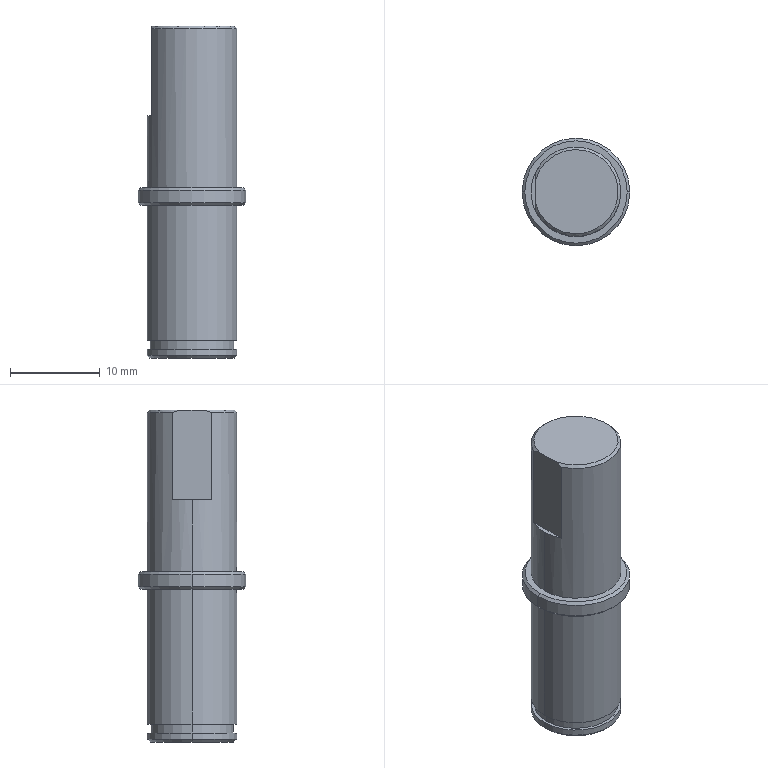Part | SolidWorks | features ICE 3, Chamfer 1, Extrusion 1, RevCut 1 | 1 solid | 25 faces | box 12 x 12 x 37 mm | volume 2944 mm3 | cylinder 10 | plane 8 | cone 7 | commonest cylinder face diameters 10 x6 9.3 x2 12 x2
STEP:
#1=CARTESIAN_POINT('',(-5.7,0.,-2.));
#2=VERTEX_POINT('',#1);
#3=CARTESIAN_POINT('',(5.7,0.,-2.));
#4=VERTEX_POINT('',#3);
#5=CARTESIAN_POINT('',(0.,0.,-2.));
#6=DIRECTION('',(0.,0.,-1.));
#7=DIRECTION('',(-1.,0.,0.));
#8=AXIS2_PLACEMENT_3D('',#5,#6,#7);
#9=CIRCLE('',#8,5.7);
#10=EDGE_CURVE('',#2,#4,#9,.T.);
#11=ORIENTED_EDGE('',*,*,#10,.F.);
#12=CARTESIAN_POINT('',(-6.,0.,-1.7));
#13=VERTEX_POINT('',#12);
#14=CARTESIAN_POINT('',(-5.7,0.,-2.));
#15=DIRECTION('',(-0.7071,0.,0.7071));
#16=VECTOR('',#15,1000.);
#17=LINE('',#14,#16);
#18=EDGE_CURVE('',#2,#13,#17,.T.);
#19=ORIENTED_EDGE('',*,*,#18,.T.);
#20=CARTESIAN_POINT('',(6.,0.,-1.7));
#21=VERTEX_POINT('',#20);
#22=CARTESIAN_POINT('',(0.,0.,-1.7));
#23=DIRECTION('',(0.,0.,1.));
#24=DIRECTION('',(-1.,0.,0.));
#25=AXIS2_PLACEMENT_3D('',#22,#23,#24);
#26=CIRCLE('',#25,6.);
#27=EDGE_CURVE('',#21,#13,#26,.T.);
#28=ORIENTED_EDGE('',*,*,#27,.F.);
#29=CARTESIAN_POINT('',(5.7,0.,-2.));
#30=DIRECTION('',(0.7071,0.,0.7071));
#31=VECTOR('',#30,1000.);
#32=LINE('',#29,#31);
#33=EDGE_CURVE('',#4,#21,#32,.T.);
#34=ORIENTED_EDGE('',*,*,#33,.F.);
#35=EDGE_LOOP('',(#11,#19,#28,#34));
#36=FACE_OUTER_BOUND('',#35,.T.);
#37=CARTESIAN_POINT('',(0.,0.,-2.));
#38=DIRECTION('',(0.,0.,1.));
#39=DIRECTION('',(1.,0.,0.));
#40=AXIS2_PLACEMENT_3D('',#37,#38,#39);
#41=CONICAL_SURFACE('',#40,5.7,0.7854);
#42=ADVANCED_FACE('',(#36),#41,.T.);
#43=CARTESIAN_POINT('',(5.7,0.,0.));
#44=VERTEX_POINT('',#43);
#45=CARTESIAN_POINT('',(-5.7,0.,0.));
#46=VERTEX_POINT('',#45);
#47=CARTESIAN_POINT('',(0.,0.,0.));
#48=DIRECTION('',(0.,0.,1.));
#49=DIRECTION('',(-1.,0.,0.));
#50=AXIS2_PLACEMENT_3D('',#47,#48,#49);
#51=CIRCLE('',#50,5.7);
#52=EDGE_CURVE('',#44,#46,#51,.T.);
#53=ORIENTED_EDGE('',*,*,#52,.F.);
#54=CARTESIAN_POINT('',(6.,0.,-0.3));
#55=VERTEX_POINT('',#54);
#56=CARTESIAN_POINT('',(6.,0.,-0.3));
#57=DIRECTION('',(0.7071,0.,-0.7071));
#58=VECTOR('',#57,1000.);
#59=LINE('',#56,#58);
#60=EDGE_CURVE('',#44,#55,#59,.T.);
#61=ORIENTED_EDGE('',*,*,#60,.T.);
#62=CARTESIAN_POINT('',(-6.,0.,-0.3));
#63=VERTEX_POINT('',#62);
#64=CARTESIAN_POINT('',(0.,0.,-0.3));
#65=DIRECTION('',(0.,0.,-1.));
#66=DIRECTION('',(-1.,0.,0.));
#67=AXIS2_PLACEMENT_3D('',#64,#65,#66);
#68=CIRCLE('',#67,6.);
#69=EDGE_CURVE('',#63,#55,#68,.T.);
#70=ORIENTED_EDGE('',*,*,#69,.F.);
#71=CARTESIAN_POINT('',(-6.,0.,-0.3));
#72=DIRECTION('',(-0.7071,0.,-0.7071));
#73=VECTOR('',#72,1000.);
#74=LINE('',#71,#73);
#75=EDGE_CURVE('',#46,#63,#74,.T.);
#76=ORIENTED_EDGE('',*,*,#75,.F.);
#77=EDGE_LOOP('',(#53,#61,#70,#76));
#78=FACE_OUTER_BOUND('',#77,.T.);
#79=CARTESIAN_POINT('',(0.,0.,-0.3));
#80=DIRECTION('',(0.,0.,-1.));
#81=DIRECTION('',(-1.,0.,0.));
#82=AXIS2_PLACEMENT_3D('',#79,#80,#81);
#83=CONICAL_SURFACE('',#82,6.,0.7854);
#84=ADVANCED_FACE('',(#78),#83,.T.);
#85=CARTESIAN_POINT('',(-4.7,0.,-19.));
#86=VERTEX_POINT('',#85);
#87=CARTESIAN_POINT('',(4.7,0.,-19.));
#88=VERTEX_POINT('',#87);
#89=CARTESIAN_POINT('',(0.,0.,-19.));
#90=DIRECTION('',(0.,0.,-1.));
#91=DIRECTION('',(-1.,0.,0.));
#92=AXIS2_PLACEMENT_3D('',#89,#90,#91);
#93=CIRCLE('',#92,4.7);
#94=EDGE_CURVE('',#86,#88,#93,.T.);
#95=ORIENTED_EDGE('',*,*,#94,.F.);
#96=CARTESIAN_POINT('',(-5.,0.,-18.7));
#97=VERTEX_POINT('',#96);
#98=CARTESIAN_POINT('',(-4.7,0.,-19.));
#99=DIRECTION('',(-0.7071,0.,0.7071));
#100=VECTOR('',#99,1000.);
#101=LINE('',#98,#100);
#102=EDGE_CURVE('',#86,#97,#101,.T.);
#103=ORIENTED_EDGE('',*,*,#102,.T.);
#104=CARTESIAN_POINT('',(5.,0.,-18.7));
#105=VERTEX_POINT('',#104);
#106=CARTESIAN_POINT('',(0.,0.,-18.7));
#107=DIRECTION('',(0.,0.,1.));
#108=DIRECTION('',(-1.,0.,0.));
#109=AXIS2_PLACEMENT_3D('',#106,#107,#108);
#110=CIRCLE('',#109,5.);
#111=EDGE_CURVE('',#105,#97,#110,.T.);
#112=ORIENTED_EDGE('',*,*,#111,.F.);
#113=CARTESIAN_POINT('',(4.7,0.,-19.));
#114=DIRECTION('',(0.7071,0.,0.7071));
#115=VECTOR('',#114,1000.);
#116=LINE('',#113,#115);
#117=EDGE_CURVE('',#88,#105,#116,.T.);
#118=ORIENTED_EDGE('',*,*,#117,.F.);
#119=EDGE_LOOP('',(#95,#103,#112,#118));
#120=FACE_OUTER_BOUND('',#119,.T.);
#121=CARTESIAN_POINT('',(0.,0.,-19.));
#122=DIRECTION('',(0.,0.,1.));
#123=DIRECTION('',(1.,0.,0.));
#124=AXIS2_PLACEMENT_3D('',#121,#122,#123);
#125=CONICAL_SURFACE('',#124,4.7,0.7854);
#126=ADVANCED_FACE('',(#120),#125,.T.);
#127=ORIENTED_EDGE('',*,*,#111,.T.);
#128=CARTESIAN_POINT('',(-5.,0.,-18.));
#129=VERTEX_POINT('',#128);
#130=CARTESIAN_POINT('',(-5.,0.,-19.));
#131=DIRECTION('',(0.,0.,1.));
#132=VECTOR('',#131,1000.);
#133=LINE('',#130,#132);
#134=EDGE_CURVE('',#97,#129,#133,.T.);
#135=ORIENTED_EDGE('',*,*,#134,.T.);
#136=CARTESIAN_POINT('',(5.,0.,-18.));
#137=VERTEX_POINT('',#136);
#138=CARTESIAN_POINT('',(0.,0.,-18.));
#139=DIRECTION('',(0.,0.,-1.));
#140=DIRECTION('',(-1.,0.,0.));
#141=AXIS2_PLACEMENT_3D('',#138,#139,#140);
#142=CIRCLE('',#141,5.);
#143=EDGE_CURVE('',#129,#137,#142,.T.);
#144=ORIENTED_EDGE('',*,*,#143,.T.);
#145=CARTESIAN_POINT('',(5.,0.,-19.));
#146=DIRECTION('',(0.,0.,1.));
#147=VECTOR('',#146,1000.);
#148=LINE('',#145,#147);
#149=EDGE_CURVE('',#105,#137,#148,.T.);
#150=ORIENTED_EDGE('',*,*,#149,.F.);
#151=EDGE_LOOP('',(#127,#135,#144,#150));
#152=FACE_OUTER_BOUND('',#151,.T.);
#153=CARTESIAN_POINT('',(0.,0.,-19.));
#154=DIRECTION('',(0.,0.,1.));
#155=DIRECTION('',(1.,0.,0.));
#156=AXIS2_PLACEMENT_3D('',#153,#154,#155);
#157=CYLINDRICAL_SURFACE('',#156,5.);
#158=ADVANCED_FACE('',(#152),#157,.T.);
#159=CARTESIAN_POINT('',(-4.65,0.,-17.));
#160=VERTEX_POINT('',#159);
#161=CARTESIAN_POINT('',(4.65,0.,-17.));
#162=VERTEX_POINT('',#161);
#163=CARTESIAN_POINT('',(0.,0.,-17.));
#164=DIRECTION('',(0.,0.,-1.));
#165=DIRECTION('',(-1.,0.,0.));
#166=AXIS2_PLACEMENT_3D('',#163,#164,#165);
#167=CIRCLE('',#166,4.65);
#168=EDGE_CURVE('',#160,#162,#167,.T.);
#169=ORIENTED_EDGE('',*,*,#168,.T.);
#170=CARTESIAN_POINT('',(4.65,0.,-18.));
#171=VERTEX_POINT('',#170);
#172=CARTESIAN_POINT('',(4.65,0.,-19.));
#173=DIRECTION('',(0.,0.,-1.));
#174=VECTOR('',#173,1000.);
#175=LINE('',#172,#174);
#176=EDGE_CURVE('',#162,#171,#175,.T.);
#177=ORIENTED_EDGE('',*,*,#176,.T.);
#178=CARTESIAN_POINT('',(-4.65,0.,-18.));
#179=VERTEX_POINT('',#178);
#180=CARTESIAN_POINT('',(0.,0.,-18.));
#181=DIRECTION('',(0.,0.,-1.));
#182=DIRECTION('',(-1.,0.,0.));
#183=AXIS2_PLACEMENT_3D('',#180,#181,#182);
#184=CIRCLE('',#183,4.65);
#185=EDGE_CURVE('',#179,#171,#184,.T.);
#186=ORIENTED_EDGE('',*,*,#185,.F.);
#187=CARTESIAN_POINT('',(-4.65,0.,-19.));
#188=DIRECTION('',(0.,0.,-1.));
#189=VECTOR('',#188,1000.);
#190=LINE('',#187,#189);
#191=EDGE_CURVE('',#160,#179,#190,.T.);
#192=ORIENTED_EDGE('',*,*,#191,.F.);
#193=EDGE_LOOP('',(#169,#177,#186,#192));
#194=FACE_OUTER_BOUND('',#193,.T.);
#195=CARTESIAN_POINT('',(0.,0.,-19.));
#196=DIRECTION('',(0.,0.,-1.));
#197=DIRECTION('',(-1.,0.,0.));
#198=AXIS2_PLACEMENT_3D('',#195,#196,#197);
#199=CYLINDRICAL_SURFACE('',#198,4.65);
#200=ADVANCED_FACE('',(#194),#199,.T.);
#201=ORIENTED_EDGE('',*,*,#27,.T.);
#202=CARTESIAN_POINT('',(-6.,0.,-2.));
#203=DIRECTION('',(0.,0.,1.));
#204=VECTOR('',#203,1000.);
#205=LINE('',#202,#204);
#206=EDGE_CURVE('',#13,#63,#205,.T.);
#207=ORIENTED_EDGE('',*,*,#206,.T.);
#208=ORIENTED_EDGE('',*,*,#69,.T.);
#209=CARTESIAN_POINT('',(6.,0.,-2.));
#210=DIRECTION('',(0.,0.,1.));
#211=VECTOR('',#210,1000.);
#212=LINE('',#209,#211);
#213=EDGE_CURVE('',#21,#55,#212,.T.);
#214=ORIENTED_EDGE('',*,*,#213,.F.);
#215=EDGE_LOOP('',(#201,#207,#208,#214));
#216=FACE_OUTER_BOUND('',#215,.T.);
#217=CARTESIAN_POINT('',(0.,0.,-2.));
#218=DIRECTION('',(0.,0.,1.));
#219=DIRECTION('',(1.,0.,0.));
#220=AXIS2_PLACEMENT_3D('',#217,#218,#219);
#221=CYLINDRICAL_SURFACE('',#220,6.);
#222=ADVANCED_FACE('',(#216),#221,.T.);
#223=CARTESIAN_POINT('',(5.,0.,-17.));
#224=VERTEX_POINT('',#223);
#225=CARTESIAN_POINT('',(-5.,0.,-17.));
#226=VERTEX_POINT('',#225);
#227=CARTESIAN_POINT('',(0.,0.,-17.));
#228=DIRECTION('',(0.,0.,1.));
#229=DIRECTION('',(1.,0.,0.));
#230=AXIS2_PLACEMENT_3D('',#227,#228,#229);
#231=CIRCLE('',#230,5.);
#232=EDGE_CURVE('',#224,#226,#231,.T.);
#233=ORIENTED_EDGE('',*,*,#232,.T.);
#234=CARTESIAN_POINT('',(-5.,0.,-2.));
#235=VERTEX_POINT('',#234);
#236=CARTESIAN_POINT('',(-5.,0.,-19.));
#237=DIRECTION('',(0.,0.,1.));
#238=VECTOR('',#237,1000.);
#239=LINE('',#236,#238);
#240=EDGE_CURVE('',#226,#235,#239,.T.);
#241=ORIENTED_EDGE('',*,*,#240,.T.);
#242=CARTESIAN_POINT('',(5.,0.,-2.));
#243=VERTEX_POINT('',#242);
#244=CARTESIAN_POINT('',(0.,0.,-2.));
#245=DIRECTION('',(0.,0.,-1.));
#246=DIRECTION('',(-1.,0.,0.));
#247=AXIS2_PLACEMENT_3D('',#244,#245,#246);
#248=CIRCLE('',#247,5.);
#249=EDGE_CURVE('',#235,#243,#248,.T.);
#250=ORIENTED_EDGE('',*,*,#249,.T.);
#251=CARTESIAN_POINT('',(5.,0.,-19.));
#252=DIRECTION('',(0.,0.,1.));
#253=VECTOR('',#252,1000.);
#254=LINE('',#251,#253);
#255=EDGE_CURVE('',#224,#243,#254,.T.);
#256=ORIENTED_EDGE('',*,*,#255,.F.);
#257=EDGE_LOOP('',(#233,#241,#250,#256));
#258=FACE_OUTER_BOUND('',#257,.T.);
#259=CARTESIAN_POINT('',(0.,0.,-19.));
#260=DIRECTION('',(0.,0.,1.));
#261=DIRECTION('',(1.,0.,0.));
#262=AXIS2_PLACEMENT_3D('',#259,#260,#261);
#263=CYLINDRICAL_SURFACE('',#262,5.);
#264=ADVANCED_FACE('',(#258),#263,.T.);
#265=CARTESIAN_POINT('',(-4.5,2.179,17.7));
#266=VERTEX_POINT('',#265);
#267=CARTESIAN_POINT('',(5.,0.,17.7));
#268=VERTEX_POINT('',#267);
#269=CARTESIAN_POINT('',(0.,0.,17.7));
#270=DIRECTION('',(0.,0.,-1.));
#271=DIRECTION('',(1.,0.,0.));
#272=AXIS2_PLACEMENT_3D('',#269,#270,#271);
#273=CIRCLE('',#272,5.);
#274=EDGE_CURVE('',#266,#268,#273,.T.);
#275=ORIENTED_EDGE('',*,*,#274,.T.);
#276=CARTESIAN_POINT('',(5.,0.,0.));
#277=VERTEX_POINT('',#276);
#278=CARTESIAN_POINT('',(5.,0.,18.));
#279=DIRECTION('',(0.,0.,-1.));
#280=VECTOR('',#279,1000.);
#281=LINE('',#278,#280);
#282=EDGE_CURVE('',#268,#277,#281,.T.);
#283=ORIENTED_EDGE('',*,*,#282,.T.);
#284=CARTESIAN_POINT('',(-5.,0.,0.));
#285=VERTEX_POINT('',#284);
#286=CARTESIAN_POINT('',(0.,0.,0.));
#287=DIRECTION('',(0.,0.,-1.));
#288=DIRECTION('',(-1.,0.,0.));
#289=AXIS2_PLACEMENT_3D('',#286,#287,#288);
#290=CIRCLE('',#289,5.);
#291=EDGE_CURVE('',#285,#277,#290,.T.);
#292=ORIENTED_EDGE('',*,*,#291,.F.);
#293=CARTESIAN_POINT('',(-5.,0.,8.));
#294=VERTEX_POINT('',#293);
#295=CARTESIAN_POINT('',(-5.,0.,18.));
#296=DIRECTION('',(0.,0.,-1.));
#297=VECTOR('',#296,1000.);
#298=LINE('',#295,#297);
#299=EDGE_CURVE('',#294,#285,#298,.T.);
#300=ORIENTED_EDGE('',*,*,#299,.F.);
#301=CARTESIAN_POINT('',(-4.5,2.179,8.));
#302=VERTEX_POINT('',#301);
#303=CARTESIAN_POINT('',(0.,0.,8.));
#304=DIRECTION('',(0.,0.,1.));
#305=DIRECTION('',(1.,0.,0.));
#306=AXIS2_PLACEMENT_3D('',#303,#304,#305);
#307=CIRCLE('',#306,5.);
#308=EDGE_CURVE('',#302,#294,#307,.T.);
#309=ORIENTED_EDGE('',*,*,#308,.F.);
#310=CARTESIAN_POINT('',(-4.5,2.179,18.));
#311=DIRECTION('',(0.,0.,-1.));
#312=VECTOR('',#311,1000.);
#313=LINE('',#310,#312);
#314=EDGE_CURVE('',#266,#302,#313,.T.);
#315=ORIENTED_EDGE('',*,*,#314,.F.);
#316=EDGE_LOOP('',(#275,#283,#292,#300,#309,#315));
#317=FACE_OUTER_BOUND('',#316,.T.);
#318=CARTESIAN_POINT('',(0.,0.,18.));
#319=DIRECTION('',(0.,0.,-1.));
#320=DIRECTION('',(-1.,0.,0.));
#321=AXIS2_PLACEMENT_3D('',#318,#319,#320);
#322=CYLINDRICAL_SURFACE('',#321,5.);
#323=ADVANCED_FACE('',(#317),#322,.T.);
#324=ORIENTED_EDGE('',*,*,#282,.F.);
#325=CARTESIAN_POINT('',(-4.5,-2.179,17.7));
#326=VERTEX_POINT('',#325);
#327=CARTESIAN_POINT('',(0.,0.,17.7));
#328=DIRECTION('',(0.,0.,-1.));
#329=DIRECTION('',(1.,0.,0.));
#330=AXIS2_PLACEMENT_3D('',#327,#328,#329);
#331=CIRCLE('',#330,5.);
#332=EDGE_CURVE('',#268,#326,#331,.T.);
#333=ORIENTED_EDGE('',*,*,#332,.T.);
#334=CARTESIAN_POINT('',(-4.5,-2.179,8.));
#335=VERTEX_POINT('',#334);
#336=CARTESIAN_POINT('',(-4.5,-2.179,18.));
#337=DIRECTION('',(0.,0.,1.));
#338=VECTOR('',#337,1000.);
#339=LINE('',#336,#338);
#340=EDGE_CURVE('',#335,#326,#339,.T.);
#341=ORIENTED_EDGE('',*,*,#340,.F.);
#342=CARTESIAN_POINT('',(0.,0.,8.));
#343=DIRECTION('',(0.,0.,1.));
#344=DIRECTION('',(1.,0.,0.));
#345=AXIS2_PLACEMENT_3D('',#342,#343,#344);
#346=CIRCLE('',#345,5.);
#347=EDGE_CURVE('',#294,#335,#346,.T.);
#348=ORIENTED_EDGE('',*,*,#347,.F.);
#349=ORIENTED_EDGE('',*,*,#299,.T.);
#350=CARTESIAN_POINT('',(0.,0.,0.));
#351=DIRECTION('',(0.,0.,-1.));
#352=DIRECTION('',(-1.,0.,0.));
#353=AXIS2_PLACEMENT_3D('',#350,#351,#352);
#354=CIRCLE('',#353,5.);
#355=EDGE_CURVE('',#277,#285,#354,.T.);
#356=ORIENTED_EDGE('',*,*,#355,.F.);
#357=EDGE_LOOP('',(#324,#333,#341,#348,#349,#356));
#358=FACE_OUTER_BOUND('',#357,.T.);
#359=CARTESIAN_POINT('',(0.,0.,18.));
#360=DIRECTION('',(0.,0.,-1.));
#361=DIRECTION('',(-1.,0.,0.));
#362=AXIS2_PLACEMENT_3D('',#359,#360,#361);
#363=CYLINDRICAL_SURFACE('',#362,5.);
#364=ADVANCED_FACE('',(#358),#363,.T.);
#365=CARTESIAN_POINT('',(-4.5,1.356,18.));
#366=VERTEX_POINT('',#365);
#367=CARTESIAN_POINT('',(-4.5,-1.356,18.));
#368=VERTEX_POINT('',#367);
#369=CARTESIAN_POINT('',(-4.5,0.,18.));
#370=DIRECTION('',(0.,-1.,0.));
#371=VECTOR('',#370,1000.);
#372=LINE('',#369,#371);
#373=EDGE_CURVE('',#366,#368,#372,.T.);
#374=ORIENTED_EDGE('',*,*,#373,.T.);
#375=CARTESIAN_POINT('',(0.,0.,18.));
#376=DIRECTION('',(0.,0.,1.));
#377=DIRECTION('',(1.,0.,0.));
#378=AXIS2_PLACEMENT_3D('',#375,#376,#377);
#379=CIRCLE('',#378,4.7);
#380=EDGE_CURVE('',#368,#366,#379,.T.);
#381=ORIENTED_EDGE('',*,*,#380,.T.);
#382=EDGE_LOOP('',(#374,#381));
#383=FACE_OUTER_BOUND('',#382,.T.);
#384=CARTESIAN_POINT('',(0.,0.,18.));
#385=DIRECTION('',(0.,0.,1.));
#386=DIRECTION('',(1.,0.,0.));
#387=AXIS2_PLACEMENT_3D('',#384,#385,#386);
#388=PLANE('',#387);
#389=ADVANCED_FACE('',(#383),#388,.T.);
#390=ORIENTED_EDGE('',*,*,#240,.F.);
#391=CARTESIAN_POINT('',(0.,0.,-17.));
#392=DIRECTION('',(0.,0.,1.));
#393=DIRECTION('',(1.,0.,0.));
#394=AXIS2_PLACEMENT_3D('',#391,#392,#393);
#395=CIRCLE('',#394,5.);
#396=EDGE_CURVE('',#226,#224,#395,.T.);
#397=ORIENTED_EDGE('',*,*,#396,.T.);
#398=ORIENTED_EDGE('',*,*,#255,.T.);
#399=CARTESIAN_POINT('',(0.,0.,-2.));
#400=DIRECTION('',(0.,0.,-1.));
#401=DIRECTION('',(-1.,0.,0.));
#402=AXIS2_PLACEMENT_3D('',#399,#400,#401);
#403=CIRCLE('',#402,5.);
#404=EDGE_CURVE('',#243,#235,#403,.T.);
#405=ORIENTED_EDGE('',*,*,#404,.T.);
#406=EDGE_LOOP('',(#390,#397,#398,#405));
#407=FACE_OUTER_BOUND('',#406,.T.);
#408=CARTESIAN_POINT('',(0.,0.,-19.));
#409=DIRECTION('',(0.,0.,1.));
#410=DIRECTION('',(1.,0.,0.));
#411=AXIS2_PLACEMENT_3D('',#408,#409,#410);
#412=CYLINDRICAL_SURFACE('',#411,5.);
#413=ADVANCED_FACE('',(#407),#412,.T.);
#414=CARTESIAN_POINT('',(0.,0.,-2.));
#415=DIRECTION('',(0.,0.,-1.));
#416=DIRECTION('',(-1.,0.,0.));
#417=AXIS2_PLACEMENT_3D('',#414,#415,#416);
#418=CIRCLE('',#417,5.7);
#419=EDGE_CURVE('',#4,#2,#418,.T.);
#420=ORIENTED_EDGE('',*,*,#419,.T.);
#421=ORIENTED_EDGE('',*,*,#10,.T.);
#422=EDGE_LOOP('',(#420,#421));
#423=FACE_OUTER_BOUND('',#422,.T.);
#424=ORIENTED_EDGE('',*,*,#404,.F.);
#425=ORIENTED_EDGE('',*,*,#249,.F.);
#426=EDGE_LOOP('',(#424,#425));
#427=FACE_BOUND('',#426,.T.);
#428=CARTESIAN_POINT('',(0.,0.,-2.));
#429=DIRECTION('',(0.,0.,-1.));
#430=DIRECTION('',(-1.,0.,0.));
#431=AXIS2_PLACEMENT_3D('',#428,#429,#430);
#432=PLANE('',#431);
#433=ADVANCED_FACE('',(#423,#427),#432,.T.);
#434=CARTESIAN_POINT('',(0.,0.,0.));
#435=DIRECTION('',(0.,0.,1.));
#436=DIRECTION('',(-1.,0.,0.));
#437=AXIS2_PLACEMENT_3D('',#434,#435,#436);
#438=CIRCLE('',#437,5.7);
#439=EDGE_CURVE('',#46,#44,#438,.T.);
#440=ORIENTED_EDGE('',*,*,#439,.T.);
#441=ORIENTED_EDGE('',*,*,#52,.T.);
#442=EDGE_LOOP('',(#440,#441));
#443=FACE_OUTER_BOUND('',#442,.T.);
#444=ORIENTED_EDGE('',*,*,#291,.T.);
#445=ORIENTED_EDGE('',*,*,#355,.T.);
#446=EDGE_LOOP('',(#444,#445));
#447=FACE_BOUND('',#446,.T.);
#448=CARTESIAN_POINT('',(0.,0.,0.));
#449=DIRECTION('',(0.,0.,-1.));
#450=DIRECTION('',(-1.,0.,0.));
#451=AXIS2_PLACEMENT_3D('',#448,#449,#450);
#452=PLANE('',#451);
#453=ADVANCED_FACE('',(#443,#447),#452,.F.);
#454=ORIENTED_EDGE('',*,*,#206,.F.);
#455=CARTESIAN_POINT('',(0.,0.,-1.7));
#456=DIRECTION('',(0.,0.,1.));
#457=DIRECTION('',(-1.,0.,0.));
#458=AXIS2_PLACEMENT_3D('',#455,#456,#457);
#459=CIRCLE('',#458,6.);
#460=EDGE_CURVE('',#13,#21,#459,.T.);
#461=ORIENTED_EDGE('',*,*,#460,.T.);
#462=ORIENTED_EDGE('',*,*,#213,.T.);
#463=CARTESIAN_POINT('',(0.,0.,-0.3));
#464=DIRECTION('',(0.,0.,-1.));
#465=DIRECTION('',(-1.,0.,0.));
#466=AXIS2_PLACEMENT_3D('',#463,#464,#465);
#467=CIRCLE('',#466,6.);
#468=EDGE_CURVE('',#55,#63,#467,.T.);
#469=ORIENTED_EDGE('',*,*,#468,.T.);
#470=EDGE_LOOP('',(#454,#461,#462,#469));
#471=FACE_OUTER_BOUND('',#470,.T.);
#472=CARTESIAN_POINT('',(0.,0.,-2.));
#473=DIRECTION('',(0.,0.,1.));
#474=DIRECTION('',(1.,0.,0.));
#475=AXIS2_PLACEMENT_3D('',#472,#473,#474);
#476=CYLINDRICAL_SURFACE('',#475,6.);
#477=ADVANCED_FACE('',(#471),#476,.T.);
#478=ORIENTED_EDGE('',*,*,#168,.F.);
#479=CARTESIAN_POINT('',(0.,0.,-17.));
#480=DIRECTION('',(0.,0.,-1.));
#481=DIRECTION('',(-1.,0.,0.));
#482=AXIS2_PLACEMENT_3D('',#479,#480,#481);
#483=CIRCLE('',#482,4.65);
#484=EDGE_CURVE('',#162,#160,#483,.T.);
#485=ORIENTED_EDGE('',*,*,#484,.F.);
#486=EDGE_LOOP('',(#478,#485));
#487=FACE_BOUND('',#486,.T.);
#488=ORIENTED_EDGE('',*,*,#232,.F.);
#489=ORIENTED_EDGE('',*,*,#396,.F.);
#490=EDGE_LOOP('',(#488,#489));
#491=FACE_OUTER_BOUND('',#490,.T.);
#492=CARTESIAN_POINT('',(-6.629,0.,-17.));
#493=DIRECTION('',(0.,0.,1.));
#494=DIRECTION('',(1.,0.,0.));
#495=AXIS2_PLACEMENT_3D('',#492,#493,#494);
#496=PLANE('',#495);
#497=ADVANCED_FACE('',(#487,#491),#496,.F.);
#498=ORIENTED_EDGE('',*,*,#185,.T.);
#499=CARTESIAN_POINT('',(0.,0.,-18.));
#500=DIRECTION('',(0.,0.,-1.));
#501=DIRECTION('',(-1.,0.,0.));
#502=AXIS2_PLACEMENT_3D('',#499,#500,#501);
#503=CIRCLE('',#502,4.65);
#504=EDGE_CURVE('',#171,#179,#503,.T.);
#505=ORIENTED_EDGE('',*,*,#504,.T.);
#506=EDGE_LOOP('',(#498,#505));
#507=FACE_BOUND('',#506,.T.);
#508=CARTESIAN_POINT('',(0.,0.,-18.));
#509=DIRECTION('',(0.,0.,-1.));
#510=DIRECTION('',(-1.,0.,0.));
#511=AXIS2_PLACEMENT_3D('',#508,#509,#510);
#512=CIRCLE('',#511,5.);
#513=EDGE_CURVE('',#137,#129,#512,.T.);
#514=ORIENTED_EDGE('',*,*,#513,.F.);
#515=ORIENTED_EDGE('',*,*,#143,.F.);
#516=EDGE_LOOP('',(#514,#515));
#517=FACE_OUTER_BOUND('',#516,.T.);
#518=CARTESIAN_POINT('',(-6.629,0.,-18.));
#519=DIRECTION('',(0.,0.,-1.));
#520=DIRECTION('',(-1.,0.,0.));
#521=AXIS2_PLACEMENT_3D('',#518,#519,#520);
#522=PLANE('',#521);
#523=ADVANCED_FACE('',(#507,#517),#522,.F.);
#524=ORIENTED_EDGE('',*,*,#176,.F.);
#525=ORIENTED_EDGE('',*,*,#484,.T.);
#526=ORIENTED_EDGE('',*,*,#191,.T.);
#527=ORIENTED_EDGE('',*,*,#504,.F.);
#528=EDGE_LOOP('',(#524,#525,#526,#527));
#529=FACE_OUTER_BOUND('',#528,.T.);
#530=CARTESIAN_POINT('',(0.,0.,-19.));
#531=DIRECTION('',(0.,0.,-1.));
#532=DIRECTION('',(-1.,0.,0.));
#533=AXIS2_PLACEMENT_3D('',#530,#531,#532);
#534=CYLINDRICAL_SURFACE('',#533,4.65);
#535=ADVANCED_FACE('',(#529),#534,.T.);
#536=CARTESIAN_POINT('',(0.,0.,-19.));
#537=DIRECTION('',(0.,0.,-1.));
#538=DIRECTION('',(-1.,0.,0.));
#539=AXIS2_PLACEMENT_3D('',#536,#537,#538);
#540=CIRCLE('',#539,4.7);
#541=EDGE_CURVE('',#88,#86,#540,.T.);
#542=ORIENTED_EDGE('',*,*,#541,.T.);
#543=ORIENTED_EDGE('',*,*,#94,.T.);
#544=EDGE_LOOP('',(#542,#543));
#545=FACE_OUTER_BOUND('',#544,.T.);
#546=CARTESIAN_POINT('',(0.,0.,-19.));
#547=DIRECTION('',(0.,0.,-1.));
#548=DIRECTION('',(-1.,0.,0.));
#549=AXIS2_PLACEMENT_3D('',#546,#547,#548);
#550=PLANE('',#549);
#551=ADVANCED_FACE('',(#545),#550,.T.);
#552=ORIENTED_EDGE('',*,*,#134,.F.);
#553=CARTESIAN_POINT('',(0.,0.,-18.7));
#554=DIRECTION('',(0.,0.,1.));
#555=DIRECTION('',(-1.,0.,0.));
#556=AXIS2_PLACEMENT_3D('',#553,#554,#555);
#557=CIRCLE('',#556,5.);
#558=EDGE_CURVE('',#97,#105,#557,.T.);
#559=ORIENTED_EDGE('',*,*,#558,.T.);
#560=ORIENTED_EDGE('',*,*,#149,.T.);
#561=ORIENTED_EDGE('',*,*,#513,.T.);
#562=EDGE_LOOP('',(#552,#559,#560,#561));
#563=FACE_OUTER_BOUND('',#562,.T.);
#564=CARTESIAN_POINT('',(0.,0.,-19.));
#565=DIRECTION('',(0.,0.,1.));
#566=DIRECTION('',(1.,0.,0.));
#567=AXIS2_PLACEMENT_3D('',#564,#565,#566);
#568=CYLINDRICAL_SURFACE('',#567,5.);
#569=ADVANCED_FACE('',(#563),#568,.T.);
#570=ORIENTED_EDGE('',*,*,#308,.T.);
#571=ORIENTED_EDGE('',*,*,#347,.T.);
#572=CARTESIAN_POINT('',(-4.5,10.,8.));
#573=DIRECTION('',(0.,-1.,0.));
#574=VECTOR('',#573,1000.);
#575=LINE('',#572,#574);
#576=EDGE_CURVE('',#302,#335,#575,.T.);
#577=ORIENTED_EDGE('',*,*,#576,.F.);
#578=EDGE_LOOP('',(#570,#571,#577));
#579=FACE_OUTER_BOUND('',#578,.T.);
#580=CARTESIAN_POINT('',(-10.067,10.,8.));
#581=DIRECTION('',(0.,0.,1.));
#582=DIRECTION('',(1.,0.,0.));
#583=AXIS2_PLACEMENT_3D('',#580,#581,#582);
#584=PLANE('',#583);
#585=ADVANCED_FACE('',(#579),#584,.T.);
#586=ORIENTED_EDGE('',*,*,#373,.F.);
#587=CARTESIAN_POINT('',(-4.5,1.356,18.));
#588=CARTESIAN_POINT('',(-4.5,1.638,17.919));
#589=CARTESIAN_POINT('',(-4.5,1.911,17.817));
#590=CARTESIAN_POINT('',(-4.5,2.179,17.7));
#591=B_SPLINE_CURVE_WITH_KNOTS('',3,(#587,#588,#589,#590),.UNSPECIFIED.,.F.,.F.,(4,4),(0.,0.000876),.UNSPECIFIED.);
#592=EDGE_CURVE('',#366,#266,#591,.T.);
#593=ORIENTED_EDGE('',*,*,#592,.T.);
#594=ORIENTED_EDGE('',*,*,#314,.T.);
#595=ORIENTED_EDGE('',*,*,#576,.T.);
#596=ORIENTED_EDGE('',*,*,#340,.T.);
#597=CARTESIAN_POINT('',(-4.5,-2.179,17.7));
#598=CARTESIAN_POINT('',(-4.5,-1.911,17.817));
#599=CARTESIAN_POINT('',(-4.5,-1.638,17.919));
#600=CARTESIAN_POINT('',(-4.5,-1.356,18.));
#601=B_SPLINE_CURVE_WITH_KNOTS('',3,(#597,#598,#599,#600),.UNSPECIFIED.,.F.,.F.,(4,4),(0.,0.000876),.UNSPECIFIED.);
#602=EDGE_CURVE('',#326,#368,#601,.T.);
#603=ORIENTED_EDGE('',*,*,#602,.T.);
#604=EDGE_LOOP('',(#586,#593,#594,#595,#596,#603));
#605=FACE_OUTER_BOUND('',#604,.T.);
#606=CARTESIAN_POINT('',(-4.5,10.,8.));
#607=DIRECTION('',(-1.,0.,0.));
#608=DIRECTION('',(0.,0.,1.));
#609=AXIS2_PLACEMENT_3D('',#606,#607,#608);
#610=PLANE('',#609);
#611=ADVANCED_FACE('',(#605),#610,.T.);
#612=ORIENTED_EDGE('',*,*,#602,.F.);
#613=ORIENTED_EDGE('',*,*,#332,.F.);
#614=ORIENTED_EDGE('',*,*,#274,.F.);
#615=ORIENTED_EDGE('',*,*,#592,.F.);
#616=ORIENTED_EDGE('',*,*,#380,.F.);
#617=EDGE_LOOP('',(#612,#613,#614,#615,#616));
#618=FACE_OUTER_BOUND('',#617,.T.);
#619=CARTESIAN_POINT('',(0.,0.,18.));
#620=DIRECTION('',(0.,0.,-1.));
#621=DIRECTION('',(-1.,0.,0.));
#622=AXIS2_PLACEMENT_3D('',#619,#620,#621);
#623=CONICAL_SURFACE('',#622,4.7,0.7854);
#624=ADVANCED_FACE('',(#618),#623,.T.);
#625=ORIENTED_EDGE('',*,*,#102,.F.);
#626=ORIENTED_EDGE('',*,*,#541,.F.);
#627=ORIENTED_EDGE('',*,*,#117,.T.);
#628=ORIENTED_EDGE('',*,*,#558,.F.);
#629=EDGE_LOOP('',(#625,#626,#627,#628));
#630=FACE_OUTER_BOUND('',#629,.T.);
#631=CARTESIAN_POINT('',(0.,0.,-19.));
#632=DIRECTION('',(0.,0.,1.));
#633=DIRECTION('',(1.,0.,0.));
#634=AXIS2_PLACEMENT_3D('',#631,#632,#633);
#635=CONICAL_SURFACE('',#634,4.7,0.7854);
#636=ADVANCED_FACE('',(#630),#635,.T.);
#637=ORIENTED_EDGE('',*,*,#60,.F.);
#638=ORIENTED_EDGE('',*,*,#439,.F.);
#639=ORIENTED_EDGE('',*,*,#75,.T.);
#640=ORIENTED_EDGE('',*,*,#468,.F.);
#641=EDGE_LOOP('',(#637,#638,#639,#640));
#642=FACE_OUTER_BOUND('',#641,.T.);
#643=CARTESIAN_POINT('',(0.,0.,-0.3));
#644=DIRECTION('',(0.,0.,-1.));
#645=DIRECTION('',(-1.,0.,0.));
#646=AXIS2_PLACEMENT_3D('',#643,#644,#645);
#647=CONICAL_SURFACE('',#646,6.,0.7854);
#648=ADVANCED_FACE('',(#642),#647,.T.);
#649=ORIENTED_EDGE('',*,*,#18,.F.);
#650=ORIENTED_EDGE('',*,*,#419,.F.);
#651=ORIENTED_EDGE('',*,*,#33,.T.);
#652=ORIENTED_EDGE('',*,*,#460,.F.);
#653=EDGE_LOOP('',(#649,#650,#651,#652));
#654=FACE_OUTER_BOUND('',#653,.T.);
#655=CARTESIAN_POINT('',(0.,0.,-2.));
#656=DIRECTION('',(0.,0.,1.));
#657=DIRECTION('',(1.,0.,0.));
#658=AXIS2_PLACEMENT_3D('',#655,#656,#657);
#659=CONICAL_SURFACE('',#658,5.7,0.7854);
#660=ADVANCED_FACE('',(#654),#659,.T.);
#661=CLOSED_SHELL('',(#42,#84,#126,#158,#200,#222,#264,#323,#364,#389,#413,#433,#453,#477,#497,#523,#535,#551,#569,#585,#611,#624,#636,#648,#660));
#662=MANIFOLD_SOLID_BREP('',#661);
#663=CARTESIAN_POINT('',(0.,0.,0.));
#664=DIRECTION('',(0.,0.,1.));
#665=DIRECTION('',(1.,0.,0.));
#666=AXIS2_PLACEMENT_3D('',#663,#664,#665);
#667=(LENGTH_UNIT()NAMED_UNIT(*)SI_UNIT(.MILLI.,.METRE.));
#668=UNCERTAINTY_MEASURE_WITH_UNIT(LENGTH_MEASURE(0.00001),#667,'','');
#669=(NAMED_UNIT(*)PLANE_ANGLE_UNIT()SI_UNIT($,.RADIAN.));
#670=(NAMED_UNIT(*)SI_UNIT($,.STERADIAN.)SOLID_ANGLE_UNIT());
#671=(GEOMETRIC_REPRESENTATION_CONTEXT(3)GLOBAL_UNCERTAINTY_ASSIGNED_CONTEXT((#668))GLOBAL_UNIT_ASSIGNED_CONTEXT((#667,#669,#670))REPRESENTATION_CONTEXT('',''));
#672=ADVANCED_BREP_SHAPE_REPRESENTATION('',(#662,#666),#671);